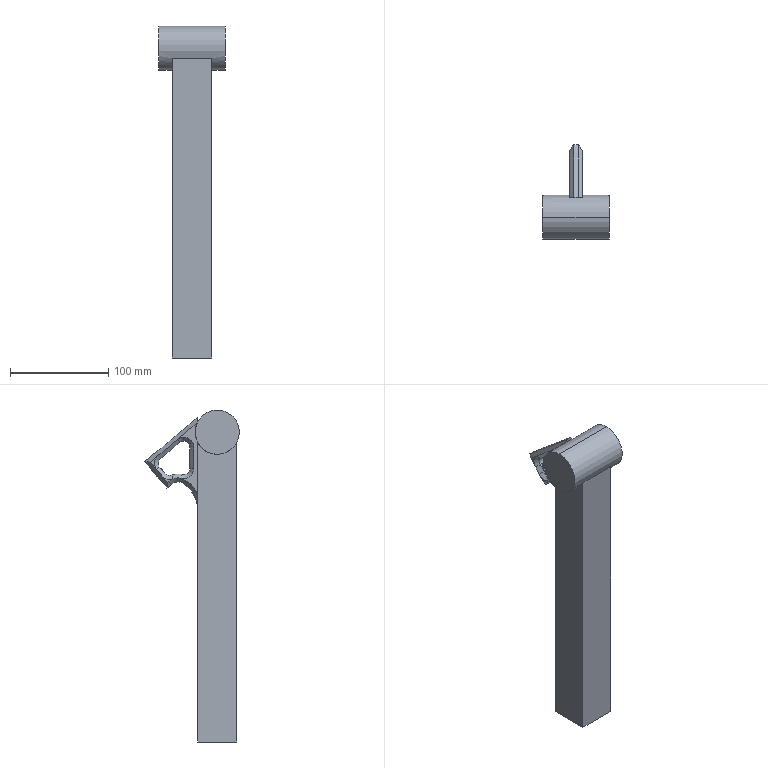Part | STEP file | Boom | 1 solid | 64 faces | box 68 x 96.123 x 337.5 mm | volume 596645 mm3 | plane 32 | cone 19 | cylinder 13 | commonest cylinder face diameters 12 x4 4.2 x2 20 x2 36 x2 45 x2 64.878 x1